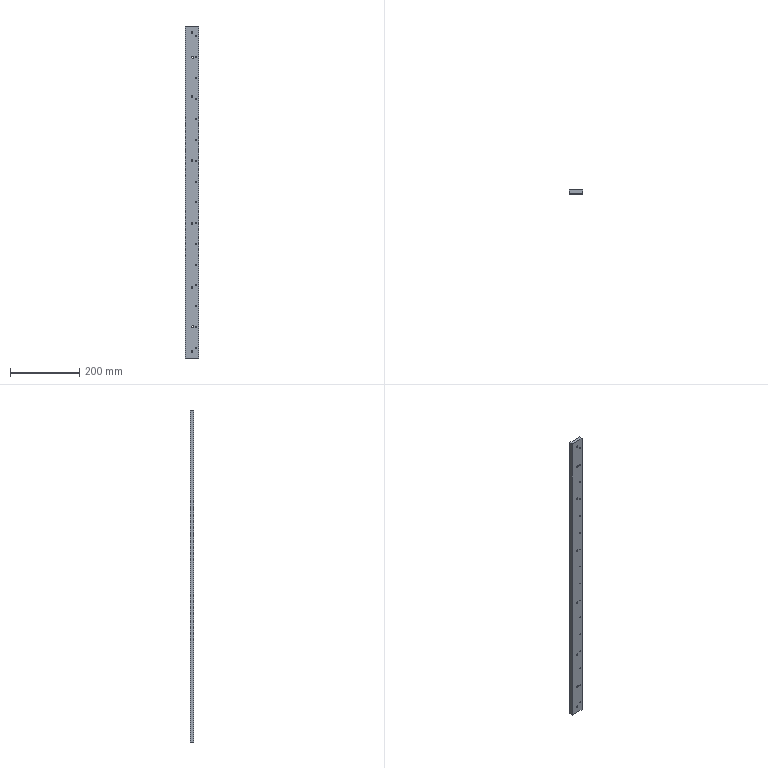Part | STEP file | 0245_220_Plate | 1 solid | 72 faces | box 40 x 10 x 960 mm | volume 379580 mm3 | cylinder 60 | plane 12 | commonest cylinder face diameters 2.5 x32 5.5 x12 10 x12 6 x4